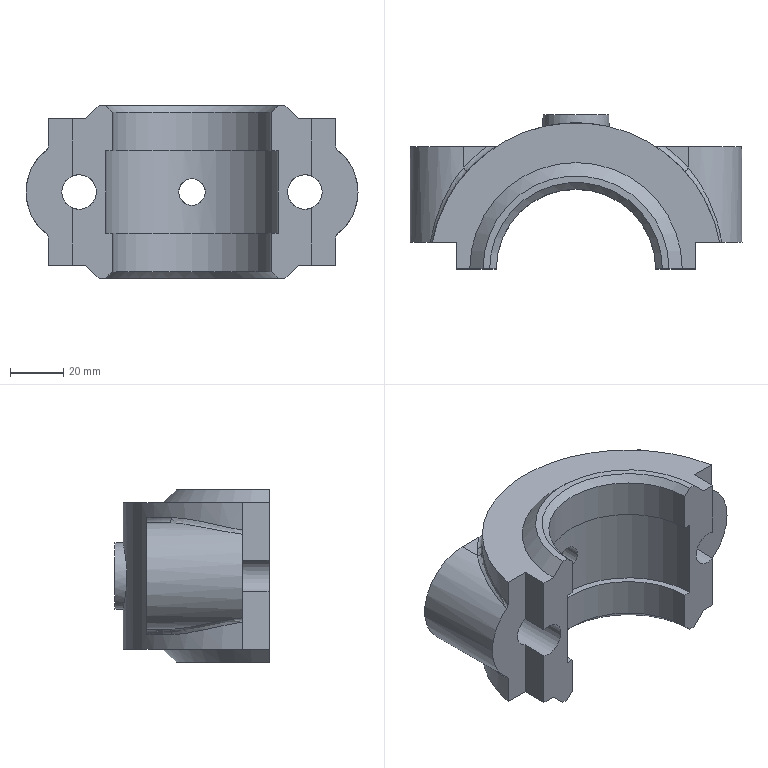Part | NX | features CHAMFER 4, HOLE PACKAGE 4, CYLINDER 3, DATUM_CSYS 3, EXTRUDE 3, SIMPLE HOLE 3, EXTRACT_STRING 2, SKETCH 2, ABSOLUTE_DATUM_PLANE 1, BLEND 1, BOSS 1, CBORE_HOLE 1, Instance Feature 1, Mirror Feature 1 | 1 solid | 45 faces | box 125 x 58 x 65 mm | volume 196230 mm3 | plane 21 | cylinder 11 | cone 5 | spline 4 | torus 4 | commonest cylinder face diameters 13 x2 40 x2 60 x2 10 x1 14 x1 25 x1